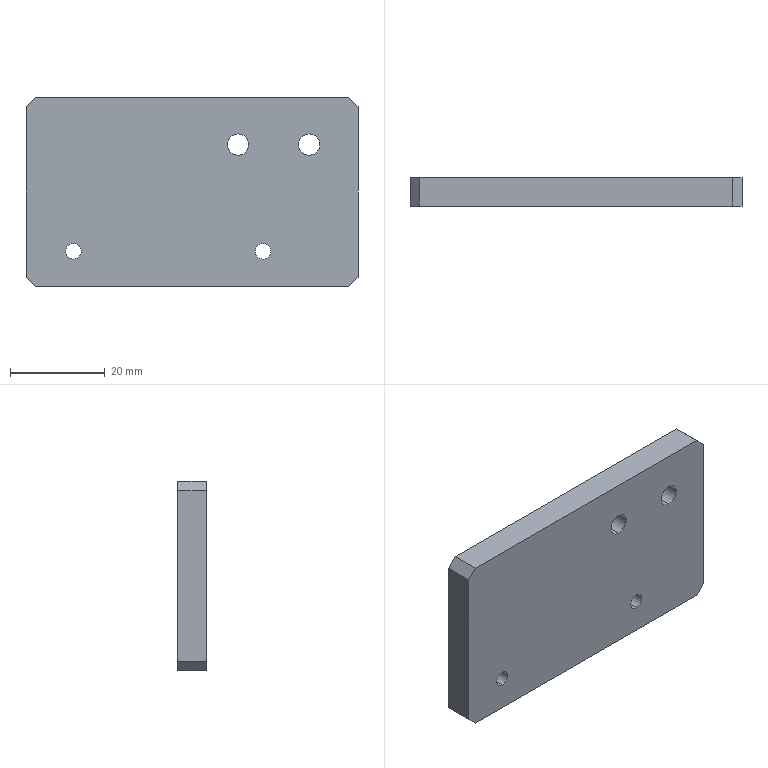Part | STEP file | PN_0023 | 1 solid | 18 faces | box 70 x 6 x 40 mm | volume 16459 mm3 | plane 10 | cylinder 8 | commonest cylinder face diameters 3.3 x4 4.5 x4
STEP:
#1=CARTESIAN_POINT('',(0.,0.,0.));
#2=DIRECTION('',(0.,0.,1.));
#3=DIRECTION('',(1.,0.,0.));
#4=AXIS2_PLACEMENT_3D('',#1,#2,#3);
#5=CARTESIAN_POINT('',(-25.,0.,-10.85));
#6=VERTEX_POINT('',#5);
#7=CARTESIAN_POINT('',(-25.,6.,-10.85));
#8=VERTEX_POINT('',#7);
#9=CARTESIAN_POINT('',(-25.,6.,-10.85));
#10=DIRECTION('',(0.,1.,0.));
#11=VECTOR('',#10,1.);
#12=LINE('',#9,#11);
#13=CARTESIAN_POINT('',(-25.,6.,-12.5));
#14=DIRECTION('',(0.,1.,0.));
#15=DIRECTION('',(0.,0.,1.));
#16=AXIS2_PLACEMENT_3D('',#13,#14,#15);
#17=CYLINDRICAL_SURFACE('',#16,1.65);
#18=CARTESIAN_POINT('',(6.283,0.));
#19=DIRECTION('',(0.,1.));
#20=VECTOR('',#19,1.);
#21=LINE('',#18,#20);
#22=(GEOMETRIC_REPRESENTATION_CONTEXT(2)PARAMETRIC_REPRESENTATION_CONTEXT()REPRESENTATION_CONTEXT('',''));
#23=DEFINITIONAL_REPRESENTATION('',(#21),#22);
#24=PCURVE('',#17,#23);
#25=CARTESIAN_POINT('',(-25.,6.,-12.5));
#26=DIRECTION('',(0.,1.,0.));
#27=DIRECTION('',(0.,0.,1.));
#28=AXIS2_PLACEMENT_3D('',#25,#26,#27);
#29=CYLINDRICAL_SURFACE('',#28,1.65);
#30=CARTESIAN_POINT('',(0.,0.));
#31=DIRECTION('',(0.,1.));
#32=VECTOR('',#31,1.);
#33=LINE('',#30,#32);
#34=(GEOMETRIC_REPRESENTATION_CONTEXT(2)PARAMETRIC_REPRESENTATION_CONTEXT()REPRESENTATION_CONTEXT('',''));
#35=DEFINITIONAL_REPRESENTATION('',(#33),#34);
#36=PCURVE('',#29,#35);
#37=SURFACE_CURVE('',#12,(#24,#36),.PCURVE_S1.);
#38=EDGE_CURVE('',#6,#8,#37,.T.);
#39=ORIENTED_EDGE('',*,*,#38,.T.);
#40=CARTESIAN_POINT('',(-25.,6.,-14.15));
#41=VERTEX_POINT('',#40);
#42=CARTESIAN_POINT('',(-25.,6.,-12.5));
#43=DIRECTION('',(0.,1.,0.));
#44=DIRECTION('',(0.,0.,1.));
#45=AXIS2_PLACEMENT_3D('',#42,#43,#44);
#46=CIRCLE('',#45,1.65);
#47=CARTESIAN_POINT('',(0.,0.));
#48=DIRECTION('',(1.,0.));
#49=VECTOR('',#48,1.);
#50=LINE('',#47,#49);
#51=(GEOMETRIC_REPRESENTATION_CONTEXT(2)PARAMETRIC_REPRESENTATION_CONTEXT()REPRESENTATION_CONTEXT('',''));
#52=DEFINITIONAL_REPRESENTATION('',(#50),#51);
#53=PCURVE('',#17,#52);
#54=CARTESIAN_POINT('',(0.,6.,0.));
#55=DIRECTION('',(0.,1.,0.));
#56=DIRECTION('',(0.,0.,1.));
#57=AXIS2_PLACEMENT_3D('',#54,#55,#56);
#58=PLANE('',#57);
#59=CARTESIAN_POINT('',(-12.5,-25.));
#60=DIRECTION('',(1.,0.));
#61=AXIS2_PLACEMENT_2D('',#59,#60);
#62=CIRCLE('',#61,1.65);
#63=(GEOMETRIC_REPRESENTATION_CONTEXT(2)PARAMETRIC_REPRESENTATION_CONTEXT()REPRESENTATION_CONTEXT('',''));
#64=DEFINITIONAL_REPRESENTATION('',(#62),#63);
#65=PCURVE('',#58,#64);
#66=SURFACE_CURVE('',#46,(#53,#65),.PCURVE_S1.);
#67=EDGE_CURVE('',#41,#8,#66,.T.);
#68=ORIENTED_EDGE('',*,*,#67,.F.);
#69=CARTESIAN_POINT('',(-25.,0.,-14.15));
#70=VERTEX_POINT('',#69);
#71=CARTESIAN_POINT('',(-25.,6.,-14.15));
#72=DIRECTION('',(0.,1.,0.));
#73=VECTOR('',#72,1.);
#74=LINE('',#71,#73);
#75=CARTESIAN_POINT('',(3.142,0.));
#76=DIRECTION('',(0.,1.));
#77=VECTOR('',#76,1.);
#78=LINE('',#75,#77);
#79=(GEOMETRIC_REPRESENTATION_CONTEXT(2)PARAMETRIC_REPRESENTATION_CONTEXT()REPRESENTATION_CONTEXT('',''));
#80=DEFINITIONAL_REPRESENTATION('',(#78),#79);
#81=PCURVE('',#17,#80);
#82=CARTESIAN_POINT('',(3.142,0.));
#83=DIRECTION('',(0.,1.));
#84=VECTOR('',#83,1.);
#85=LINE('',#82,#84);
#86=(GEOMETRIC_REPRESENTATION_CONTEXT(2)PARAMETRIC_REPRESENTATION_CONTEXT()REPRESENTATION_CONTEXT('',''));
#87=DEFINITIONAL_REPRESENTATION('',(#85),#86);
#88=PCURVE('',#29,#87);
#89=SURFACE_CURVE('',#74,(#81,#88),.PCURVE_S1.);
#90=EDGE_CURVE('',#70,#41,#89,.T.);
#91=ORIENTED_EDGE('',*,*,#90,.F.);
#92=CARTESIAN_POINT('',(-25.,0.,-12.5));
#93=DIRECTION('',(0.,1.,0.));
#94=DIRECTION('',(0.,0.,1.));
#95=AXIS2_PLACEMENT_3D('',#92,#93,#94);
#96=CIRCLE('',#95,1.65);
#97=CARTESIAN_POINT('',(0.,-6.));
#98=DIRECTION('',(1.,0.));
#99=VECTOR('',#98,1.);
#100=LINE('',#97,#99);
#101=(GEOMETRIC_REPRESENTATION_CONTEXT(2)PARAMETRIC_REPRESENTATION_CONTEXT()REPRESENTATION_CONTEXT('',''));
#102=DEFINITIONAL_REPRESENTATION('',(#100),#101);
#103=PCURVE('',#17,#102);
#104=CARTESIAN_POINT('',(0.,0.,0.));
#105=DIRECTION('',(0.,1.,0.));
#106=DIRECTION('',(0.,0.,1.));
#107=AXIS2_PLACEMENT_3D('',#104,#105,#106);
#108=PLANE('',#107);
#109=CARTESIAN_POINT('',(-12.5,-25.));
#110=DIRECTION('',(1.,0.));
#111=AXIS2_PLACEMENT_2D('',#109,#110);
#112=CIRCLE('',#111,1.65);
#113=(GEOMETRIC_REPRESENTATION_CONTEXT(2)PARAMETRIC_REPRESENTATION_CONTEXT()REPRESENTATION_CONTEXT('',''));
#114=DEFINITIONAL_REPRESENTATION('',(#112),#113);
#115=PCURVE('',#108,#114);
#116=SURFACE_CURVE('',#96,(#103,#115),.PCURVE_S1.);
#117=EDGE_CURVE('',#70,#6,#116,.T.);
#118=ORIENTED_EDGE('',*,*,#117,.T.);
#119=EDGE_LOOP('',(#39,#68,#91,#118));
#120=FACE_BOUND('',#119,.F.);
#121=ADVANCED_FACE('',(#120),#17,.F.);
#122=CARTESIAN_POINT('',(15.,0.,-10.85));
#123=VERTEX_POINT('',#122);
#124=CARTESIAN_POINT('',(15.,6.,-10.85));
#125=VERTEX_POINT('',#124);
#126=CARTESIAN_POINT('',(15.,6.,-10.85));
#127=DIRECTION('',(0.,1.,0.));
#128=VECTOR('',#127,1.);
#129=LINE('',#126,#128);
#130=CARTESIAN_POINT('',(15.,6.,-12.5));
#131=DIRECTION('',(0.,1.,0.));
#132=DIRECTION('',(0.,0.,1.));
#133=AXIS2_PLACEMENT_3D('',#130,#131,#132);
#134=CYLINDRICAL_SURFACE('',#133,1.65);
#135=CARTESIAN_POINT('',(6.283,0.));
#136=DIRECTION('',(0.,1.));
#137=VECTOR('',#136,1.);
#138=LINE('',#135,#137);
#139=(GEOMETRIC_REPRESENTATION_CONTEXT(2)PARAMETRIC_REPRESENTATION_CONTEXT()REPRESENTATION_CONTEXT('',''));
#140=DEFINITIONAL_REPRESENTATION('',(#138),#139);
#141=PCURVE('',#134,#140);
#142=CARTESIAN_POINT('',(15.,6.,-12.5));
#143=DIRECTION('',(0.,1.,0.));
#144=DIRECTION('',(0.,0.,1.));
#145=AXIS2_PLACEMENT_3D('',#142,#143,#144);
#146=CYLINDRICAL_SURFACE('',#145,1.65);
#147=CARTESIAN_POINT('',(0.,0.));
#148=DIRECTION('',(0.,1.));
#149=VECTOR('',#148,1.);
#150=LINE('',#147,#149);
#151=(GEOMETRIC_REPRESENTATION_CONTEXT(2)PARAMETRIC_REPRESENTATION_CONTEXT()REPRESENTATION_CONTEXT('',''));
#152=DEFINITIONAL_REPRESENTATION('',(#150),#151);
#153=PCURVE('',#146,#152);
#154=SURFACE_CURVE('',#129,(#141,#153),.PCURVE_S1.);
#155=EDGE_CURVE('',#123,#125,#154,.T.);
#156=ORIENTED_EDGE('',*,*,#155,.T.);
#157=CARTESIAN_POINT('',(15.,6.,-14.15));
#158=VERTEX_POINT('',#157);
#159=CARTESIAN_POINT('',(15.,6.,-12.5));
#160=DIRECTION('',(0.,1.,0.));
#161=DIRECTION('',(0.,0.,1.));
#162=AXIS2_PLACEMENT_3D('',#159,#160,#161);
#163=CIRCLE('',#162,1.65);
#164=CARTESIAN_POINT('',(0.,0.));
#165=DIRECTION('',(1.,0.));
#166=VECTOR('',#165,1.);
#167=LINE('',#164,#166);
#168=(GEOMETRIC_REPRESENTATION_CONTEXT(2)PARAMETRIC_REPRESENTATION_CONTEXT()REPRESENTATION_CONTEXT('',''));
#169=DEFINITIONAL_REPRESENTATION('',(#167),#168);
#170=PCURVE('',#134,#169);
#171=CARTESIAN_POINT('',(-12.5,15.));
#172=DIRECTION('',(1.,0.));
#173=AXIS2_PLACEMENT_2D('',#171,#172);
#174=CIRCLE('',#173,1.65);
#175=(GEOMETRIC_REPRESENTATION_CONTEXT(2)PARAMETRIC_REPRESENTATION_CONTEXT()REPRESENTATION_CONTEXT('',''));
#176=DEFINITIONAL_REPRESENTATION('',(#174),#175);
#177=PCURVE('',#58,#176);
#178=SURFACE_CURVE('',#163,(#170,#177),.PCURVE_S1.);
#179=EDGE_CURVE('',#158,#125,#178,.T.);
#180=ORIENTED_EDGE('',*,*,#179,.F.);
#181=CARTESIAN_POINT('',(15.,0.,-14.15));
#182=VERTEX_POINT('',#181);
#183=CARTESIAN_POINT('',(15.,6.,-14.15));
#184=DIRECTION('',(0.,1.,0.));
#185=VECTOR('',#184,1.);
#186=LINE('',#183,#185);
#187=CARTESIAN_POINT('',(3.142,0.));
#188=DIRECTION('',(0.,1.));
#189=VECTOR('',#188,1.);
#190=LINE('',#187,#189);
#191=(GEOMETRIC_REPRESENTATION_CONTEXT(2)PARAMETRIC_REPRESENTATION_CONTEXT()REPRESENTATION_CONTEXT('',''));
#192=DEFINITIONAL_REPRESENTATION('',(#190),#191);
#193=PCURVE('',#134,#192);
#194=CARTESIAN_POINT('',(3.142,0.));
#195=DIRECTION('',(0.,1.));
#196=VECTOR('',#195,1.);
#197=LINE('',#194,#196);
#198=(GEOMETRIC_REPRESENTATION_CONTEXT(2)PARAMETRIC_REPRESENTATION_CONTEXT()REPRESENTATION_CONTEXT('',''));
#199=DEFINITIONAL_REPRESENTATION('',(#197),#198);
#200=PCURVE('',#146,#199);
#201=SURFACE_CURVE('',#186,(#193,#200),.PCURVE_S1.);
#202=EDGE_CURVE('',#182,#158,#201,.T.);
#203=ORIENTED_EDGE('',*,*,#202,.F.);
#204=CARTESIAN_POINT('',(15.,0.,-12.5));
#205=DIRECTION('',(0.,1.,0.));
#206=DIRECTION('',(0.,0.,1.));
#207=AXIS2_PLACEMENT_3D('',#204,#205,#206);
#208=CIRCLE('',#207,1.65);
#209=CARTESIAN_POINT('',(0.,-6.));
#210=DIRECTION('',(1.,0.));
#211=VECTOR('',#210,1.);
#212=LINE('',#209,#211);
#213=(GEOMETRIC_REPRESENTATION_CONTEXT(2)PARAMETRIC_REPRESENTATION_CONTEXT()REPRESENTATION_CONTEXT('',''));
#214=DEFINITIONAL_REPRESENTATION('',(#212),#213);
#215=PCURVE('',#134,#214);
#216=CARTESIAN_POINT('',(-12.5,15.));
#217=DIRECTION('',(1.,0.));
#218=AXIS2_PLACEMENT_2D('',#216,#217);
#219=CIRCLE('',#218,1.65);
#220=(GEOMETRIC_REPRESENTATION_CONTEXT(2)PARAMETRIC_REPRESENTATION_CONTEXT()REPRESENTATION_CONTEXT('',''));
#221=DEFINITIONAL_REPRESENTATION('',(#219),#220);
#222=PCURVE('',#108,#221);
#223=SURFACE_CURVE('',#208,(#215,#222),.PCURVE_S1.);
#224=EDGE_CURVE('',#182,#123,#223,.T.);
#225=ORIENTED_EDGE('',*,*,#224,.T.);
#226=EDGE_LOOP('',(#156,#180,#203,#225));
#227=FACE_BOUND('',#226,.F.);
#228=ADVANCED_FACE('',(#227),#134,.F.);
#229=CARTESIAN_POINT('',(24.703,0.,12.25));
#230=VERTEX_POINT('',#229);
#231=CARTESIAN_POINT('',(24.703,6.,12.25));
#232=VERTEX_POINT('',#231);
#233=CARTESIAN_POINT('',(24.703,6.,12.25));
#234=DIRECTION('',(0.,1.,0.));
#235=VECTOR('',#234,1.);
#236=LINE('',#233,#235);
#237=CARTESIAN_POINT('',(24.703,6.,10.));
#238=DIRECTION('',(0.,1.,0.));
#239=DIRECTION('',(0.,0.,1.));
#240=AXIS2_PLACEMENT_3D('',#237,#238,#239);
#241=CYLINDRICAL_SURFACE('',#240,2.25);
#242=CARTESIAN_POINT('',(6.283,0.));
#243=DIRECTION('',(0.,1.));
#244=VECTOR('',#243,1.);
#245=LINE('',#242,#244);
#246=(GEOMETRIC_REPRESENTATION_CONTEXT(2)PARAMETRIC_REPRESENTATION_CONTEXT()REPRESENTATION_CONTEXT('',''));
#247=DEFINITIONAL_REPRESENTATION('',(#245),#246);
#248=PCURVE('',#241,#247);
#249=CARTESIAN_POINT('',(24.703,6.,10.));
#250=DIRECTION('',(0.,1.,0.));
#251=DIRECTION('',(0.,0.,1.));
#252=AXIS2_PLACEMENT_3D('',#249,#250,#251);
#253=CYLINDRICAL_SURFACE('',#252,2.25);
#254=CARTESIAN_POINT('',(0.,0.));
#255=DIRECTION('',(0.,1.));
#256=VECTOR('',#255,1.);
#257=LINE('',#254,#256);
#258=(GEOMETRIC_REPRESENTATION_CONTEXT(2)PARAMETRIC_REPRESENTATION_CONTEXT()REPRESENTATION_CONTEXT('',''));
#259=DEFINITIONAL_REPRESENTATION('',(#257),#258);
#260=PCURVE('',#253,#259);
#261=SURFACE_CURVE('',#236,(#248,#260),.PCURVE_S1.);
#262=EDGE_CURVE('',#230,#232,#261,.T.);
#263=ORIENTED_EDGE('',*,*,#262,.T.);
#264=CARTESIAN_POINT('',(24.703,6.,7.75));
#265=VERTEX_POINT('',#264);
#266=CARTESIAN_POINT('',(24.703,6.,10.));
#267=DIRECTION('',(0.,1.,0.));
#268=DIRECTION('',(0.,0.,1.));
#269=AXIS2_PLACEMENT_3D('',#266,#267,#268);
#270=CIRCLE('',#269,2.25);
#271=CARTESIAN_POINT('',(0.,0.));
#272=DIRECTION('',(1.,0.));
#273=VECTOR('',#272,1.);
#274=LINE('',#271,#273);
#275=(GEOMETRIC_REPRESENTATION_CONTEXT(2)PARAMETRIC_REPRESENTATION_CONTEXT()REPRESENTATION_CONTEXT('',''));
#276=DEFINITIONAL_REPRESENTATION('',(#274),#275);
#277=PCURVE('',#241,#276);
#278=CARTESIAN_POINT('',(10.,24.703));
#279=DIRECTION('',(1.,0.));
#280=AXIS2_PLACEMENT_2D('',#278,#279);
#281=CIRCLE('',#280,2.25);
#282=(GEOMETRIC_REPRESENTATION_CONTEXT(2)PARAMETRIC_REPRESENTATION_CONTEXT()REPRESENTATION_CONTEXT('',''));
#283=DEFINITIONAL_REPRESENTATION('',(#281),#282);
#284=PCURVE('',#58,#283);
#285=SURFACE_CURVE('',#270,(#277,#284),.PCURVE_S1.);
#286=EDGE_CURVE('',#265,#232,#285,.T.);
#287=ORIENTED_EDGE('',*,*,#286,.F.);
#288=CARTESIAN_POINT('',(24.703,0.,7.75));
#289=VERTEX_POINT('',#288);
#290=CARTESIAN_POINT('',(24.703,6.,7.75));
#291=DIRECTION('',(0.,1.,0.));
#292=VECTOR('',#291,1.);
#293=LINE('',#290,#292);
#294=CARTESIAN_POINT('',(3.142,0.));
#295=DIRECTION('',(0.,1.));
#296=VECTOR('',#295,1.);
#297=LINE('',#294,#296);
#298=(GEOMETRIC_REPRESENTATION_CONTEXT(2)PARAMETRIC_REPRESENTATION_CONTEXT()REPRESENTATION_CONTEXT('',''));
#299=DEFINITIONAL_REPRESENTATION('',(#297),#298);
#300=PCURVE('',#241,#299);
#301=CARTESIAN_POINT('',(3.142,0.));
#302=DIRECTION('',(0.,1.));
#303=VECTOR('',#302,1.);
#304=LINE('',#301,#303);
#305=(GEOMETRIC_REPRESENTATION_CONTEXT(2)PARAMETRIC_REPRESENTATION_CONTEXT()REPRESENTATION_CONTEXT('',''));
#306=DEFINITIONAL_REPRESENTATION('',(#304),#305);
#307=PCURVE('',#253,#306);
#308=SURFACE_CURVE('',#293,(#300,#307),.PCURVE_S1.);
#309=EDGE_CURVE('',#289,#265,#308,.T.);
#310=ORIENTED_EDGE('',*,*,#309,.F.);
#311=CARTESIAN_POINT('',(24.703,0.,10.));
#312=DIRECTION('',(0.,1.,0.));
#313=DIRECTION('',(0.,0.,1.));
#314=AXIS2_PLACEMENT_3D('',#311,#312,#313);
#315=CIRCLE('',#314,2.25);
#316=CARTESIAN_POINT('',(0.,-6.));
#317=DIRECTION('',(1.,0.));
#318=VECTOR('',#317,1.);
#319=LINE('',#316,#318);
#320=(GEOMETRIC_REPRESENTATION_CONTEXT(2)PARAMETRIC_REPRESENTATION_CONTEXT()REPRESENTATION_CONTEXT('',''));
#321=DEFINITIONAL_REPRESENTATION('',(#319),#320);
#322=PCURVE('',#241,#321);
#323=CARTESIAN_POINT('',(10.,24.703));
#324=DIRECTION('',(1.,0.));
#325=AXIS2_PLACEMENT_2D('',#323,#324);
#326=CIRCLE('',#325,2.25);
#327=(GEOMETRIC_REPRESENTATION_CONTEXT(2)PARAMETRIC_REPRESENTATION_CONTEXT()REPRESENTATION_CONTEXT('',''));
#328=DEFINITIONAL_REPRESENTATION('',(#326),#327);
#329=PCURVE('',#108,#328);
#330=SURFACE_CURVE('',#315,(#322,#329),.PCURVE_S1.);
#331=EDGE_CURVE('',#289,#230,#330,.T.);
#332=ORIENTED_EDGE('',*,*,#331,.T.);
#333=EDGE_LOOP('',(#263,#287,#310,#332));
#334=FACE_BOUND('',#333,.F.);
#335=ADVANCED_FACE('',(#334),#241,.F.);
#336=CARTESIAN_POINT('',(9.703,0.,12.25));
#337=VERTEX_POINT('',#336);
#338=CARTESIAN_POINT('',(9.703,6.,12.25));
#339=VERTEX_POINT('',#338);
#340=CARTESIAN_POINT('',(9.703,6.,12.25));
#341=DIRECTION('',(0.,1.,0.));
#342=VECTOR('',#341,1.);
#343=LINE('',#340,#342);
#344=CARTESIAN_POINT('',(9.703,6.,10.));
#345=DIRECTION('',(0.,1.,0.));
#346=DIRECTION('',(0.,0.,1.));
#347=AXIS2_PLACEMENT_3D('',#344,#345,#346);
#348=CYLINDRICAL_SURFACE('',#347,2.25);
#349=CARTESIAN_POINT('',(6.283,0.));
#350=DIRECTION('',(0.,1.));
#351=VECTOR('',#350,1.);
#352=LINE('',#349,#351);
#353=(GEOMETRIC_REPRESENTATION_CONTEXT(2)PARAMETRIC_REPRESENTATION_CONTEXT()REPRESENTATION_CONTEXT('',''));
#354=DEFINITIONAL_REPRESENTATION('',(#352),#353);
#355=PCURVE('',#348,#354);
#356=CARTESIAN_POINT('',(9.703,6.,10.));
#357=DIRECTION('',(0.,1.,0.));
#358=DIRECTION('',(0.,0.,1.));
#359=AXIS2_PLACEMENT_3D('',#356,#357,#358);
#360=CYLINDRICAL_SURFACE('',#359,2.25);
#361=CARTESIAN_POINT('',(0.,0.));
#362=DIRECTION('',(0.,1.));
#363=VECTOR('',#362,1.);
#364=LINE('',#361,#363);
#365=(GEOMETRIC_REPRESENTATION_CONTEXT(2)PARAMETRIC_REPRESENTATION_CONTEXT()REPRESENTATION_CONTEXT('',''));
#366=DEFINITIONAL_REPRESENTATION('',(#364),#365);
#367=PCURVE('',#360,#366);
#368=SURFACE_CURVE('',#343,(#355,#367),.PCURVE_S1.);
#369=EDGE_CURVE('',#337,#339,#368,.T.);
#370=ORIENTED_EDGE('',*,*,#369,.T.);
#371=CARTESIAN_POINT('',(9.703,6.,7.75));
#372=VERTEX_POINT('',#371);
#373=CARTESIAN_POINT('',(9.703,6.,10.));
#374=DIRECTION('',(0.,1.,0.));
#375=DIRECTION('',(0.,0.,1.));
#376=AXIS2_PLACEMENT_3D('',#373,#374,#375);
#377=CIRCLE('',#376,2.25);
#378=CARTESIAN_POINT('',(0.,0.));
#379=DIRECTION('',(1.,0.));
#380=VECTOR('',#379,1.);
#381=LINE('',#378,#380);
#382=(GEOMETRIC_REPRESENTATION_CONTEXT(2)PARAMETRIC_REPRESENTATION_CONTEXT()REPRESENTATION_CONTEXT('',''));
#383=DEFINITIONAL_REPRESENTATION('',(#381),#382);
#384=PCURVE('',#348,#383);
#385=CARTESIAN_POINT('',(10.,9.703));
#386=DIRECTION('',(1.,0.));
#387=AXIS2_PLACEMENT_2D('',#385,#386);
#388=CIRCLE('',#387,2.25);
#389=(GEOMETRIC_REPRESENTATION_CONTEXT(2)PARAMETRIC_REPRESENTATION_CONTEXT()REPRESENTATION_CONTEXT('',''));
#390=DEFINITIONAL_REPRESENTATION('',(#388),#389);
#391=PCURVE('',#58,#390);
#392=SURFACE_CURVE('',#377,(#384,#391),.PCURVE_S1.);
#393=EDGE_CURVE('',#372,#339,#392,.T.);
#394=ORIENTED_EDGE('',*,*,#393,.F.);
#395=CARTESIAN_POINT('',(9.703,0.,7.75));
#396=VERTEX_POINT('',#395);
#397=CARTESIAN_POINT('',(9.703,6.,7.75));
#398=DIRECTION('',(0.,1.,0.));
#399=VECTOR('',#398,1.);
#400=LINE('',#397,#399);
#401=CARTESIAN_POINT('',(3.142,0.));
#402=DIRECTION('',(0.,1.));
#403=VECTOR('',#402,1.);
#404=LINE('',#401,#403);
#405=(GEOMETRIC_REPRESENTATION_CONTEXT(2)PARAMETRIC_REPRESENTATION_CONTEXT()REPRESENTATION_CONTEXT('',''));
#406=DEFINITIONAL_REPRESENTATION('',(#404),#405);
#407=PCURVE('',#348,#406);
#408=CARTESIAN_POINT('',(3.142,0.));
#409=DIRECTION('',(0.,1.));
#410=VECTOR('',#409,1.);
#411=LINE('',#408,#410);
#412=(GEOMETRIC_REPRESENTATION_CONTEXT(2)PARAMETRIC_REPRESENTATION_CONTEXT()REPRESENTATION_CONTEXT('',''));
#413=DEFINITIONAL_REPRESENTATION('',(#411),#412);
#414=PCURVE('',#360,#413);
#415=SURFACE_CURVE('',#400,(#407,#414),.PCURVE_S1.);
#416=EDGE_CURVE('',#396,#372,#415,.T.);
#417=ORIENTED_EDGE('',*,*,#416,.F.);
#418=CARTESIAN_POINT('',(9.703,0.,10.));
#419=DIRECTION('',(0.,1.,0.));
#420=DIRECTION('',(0.,0.,1.));
#421=AXIS2_PLACEMENT_3D('',#418,#419,#420);
#422=CIRCLE('',#421,2.25);
#423=CARTESIAN_POINT('',(0.,-6.));
#424=DIRECTION('',(1.,0.));
#425=VECTOR('',#424,1.);
#426=LINE('',#423,#425);
#427=(GEOMETRIC_REPRESENTATION_CONTEXT(2)PARAMETRIC_REPRESENTATION_CONTEXT()REPRESENTATION_CONTEXT('',''));
#428=DEFINITIONAL_REPRESENTATION('',(#426),#427);
#429=PCURVE('',#348,#428);
#430=CARTESIAN_POINT('',(10.,9.703));
#431=DIRECTION('',(1.,0.));
#432=AXIS2_PLACEMENT_2D('',#430,#431);
#433=CIRCLE('',#432,2.25);
#434=(GEOMETRIC_REPRESENTATION_CONTEXT(2)PARAMETRIC_REPRESENTATION_CONTEXT()REPRESENTATION_CONTEXT('',''));
#435=DEFINITIONAL_REPRESENTATION('',(#433),#434);
#436=PCURVE('',#108,#435);
#437=SURFACE_CURVE('',#422,(#429,#436),.PCURVE_S1.);
#438=EDGE_CURVE('',#396,#337,#437,.T.);
#439=ORIENTED_EDGE('',*,*,#438,.T.);
#440=EDGE_LOOP('',(#370,#394,#417,#439));
#441=FACE_BOUND('',#440,.F.);
#442=ADVANCED_FACE('',(#441),#348,.F.);
#443=CARTESIAN_POINT('',(35.,6.,18.));
#444=VERTEX_POINT('',#443);
#445=CARTESIAN_POINT('',(35.,6.,-18.));
#446=VERTEX_POINT('',#445);
#447=CARTESIAN_POINT('',(35.,6.,-20.));
#448=DIRECTION('',(0.,0.,-1.));
#449=VECTOR('',#448,1.);
#450=LINE('',#447,#449);
#451=CARTESIAN_POINT('',(35.,6.,-20.));
#452=DIRECTION('',(-1.,0.,0.));
#453=DIRECTION('',(0.,0.,1.));
#454=AXIS2_PLACEMENT_3D('',#451,#452,#453);
#455=PLANE('',#454);
#456=CARTESIAN_POINT('',(0.,0.));
#457=DIRECTION('',(-1.,0.));
#458=VECTOR('',#457,1.);
#459=LINE('',#456,#458);
#460=(GEOMETRIC_REPRESENTATION_CONTEXT(2)PARAMETRIC_REPRESENTATION_CONTEXT()REPRESENTATION_CONTEXT('',''));
#461=DEFINITIONAL_REPRESENTATION('',(#459),#460);
#462=PCURVE('',#455,#461);
#463=CARTESIAN_POINT('',(-20.,35.));
#464=DIRECTION('',(-1.,0.));
#465=VECTOR('',#464,1.);
#466=LINE('',#463,#465);
#467=(GEOMETRIC_REPRESENTATION_CONTEXT(2)PARAMETRIC_REPRESENTATION_CONTEXT()REPRESENTATION_CONTEXT('',''));
#468=DEFINITIONAL_REPRESENTATION('',(#466),#467);
#469=PCURVE('',#58,#468);
#470=SURFACE_CURVE('',#450,(#462,#469),.PCURVE_S1.);
#471=EDGE_CURVE('',#444,#446,#470,.T.);
#472=ORIENTED_EDGE('',*,*,#471,.F.);
#473=CARTESIAN_POINT('',(35.,0.,18.));
#474=VERTEX_POINT('',#473);
#475=CARTESIAN_POINT('',(35.,6.,18.));
#476=DIRECTION('',(0.,-1.,0.));
#477=VECTOR('',#476,1.);
#478=LINE('',#475,#477);
#479=CARTESIAN_POINT('',(38.,0.));
#480=DIRECTION('',(0.,-1.));
#481=VECTOR('',#480,1.);
#482=LINE('',#479,#481);
#483=(GEOMETRIC_REPRESENTATION_CONTEXT(2)PARAMETRIC_REPRESENTATION_CONTEXT()REPRESENTATION_CONTEXT('',''));
#484=DEFINITIONAL_REPRESENTATION('',(#482),#483);
#485=PCURVE('',#455,#484);
#486=CARTESIAN_POINT('',(35.,6.,18.));
#487=DIRECTION('',(-0.7071,0.,-0.7071));
#488=DIRECTION('',(0.,-1.,0.));
#489=AXIS2_PLACEMENT_3D('',#486,#487,#488);
#490=PLANE('',#489);
#491=CARTESIAN_POINT('',(0.,0.));
#492=DIRECTION('',(1.,0.));
#493=VECTOR('',#492,1.);
#494=LINE('',#491,#493);
#495=(GEOMETRIC_REPRESENTATION_CONTEXT(2)PARAMETRIC_REPRESENTATION_CONTEXT()REPRESENTATION_CONTEXT('',''));
#496=DEFINITIONAL_REPRESENTATION('',(#494),#495);
#497=PCURVE('',#490,#496);
#498=SURFACE_CURVE('',#478,(#485,#497),.PCURVE_S1.);
#499=EDGE_CURVE('',#444,#474,#498,.T.);
#500=ORIENTED_EDGE('',*,*,#499,.T.);
#501=CARTESIAN_POINT('',(35.,0.,-18.));
#502=VERTEX_POINT('',#501);
#503=CARTESIAN_POINT('',(35.,0.,-20.));
#504=DIRECTION('',(0.,0.,-1.));
#505=VECTOR('',#504,1.);
#506=LINE('',#503,#505);
#507=CARTESIAN_POINT('',(0.,-6.));
#508=DIRECTION('',(-1.,0.));
#509=VECTOR('',#508,1.);
#510=LINE('',#507,#509);
#511=(GEOMETRIC_REPRESENTATION_CONTEXT(2)PARAMETRIC_REPRESENTATION_CONTEXT()REPRESENTATION_CONTEXT('',''));
#512=DEFINITIONAL_REPRESENTATION('',(#510),#511);
#513=PCURVE('',#455,#512);
#514=CARTESIAN_POINT('',(-20.,35.));
#515=DIRECTION('',(-1.,0.));
#516=VECTOR('',#515,1.);
#517=LINE('',#514,#516);
#518=(GEOMETRIC_REPRESENTATION_CONTEXT(2)PARAMETRIC_REPRESENTATION_CONTEXT()REPRESENTATION_CONTEXT('',''));
#519=DEFINITIONAL_REPRESENTATION('',(#517),#518);
#520=PCURVE('',#108,#519);
#521=SURFACE_CURVE('',#506,(#513,#520),.PCURVE_S1.);
#522=EDGE_CURVE('',#474,#502,#521,.T.);
#523=ORIENTED_EDGE('',*,*,#522,.T.);
#524=CARTESIAN_POINT('',(35.,6.,-18.));
#525=DIRECTION('',(0.,1.,0.));
#526=VECTOR('',#525,1.);
#527=LINE('',#524,#526);
#528=CARTESIAN_POINT('',(2.,0.));
#529=DIRECTION('',(0.,1.));
#530=VECTOR('',#529,1.);
#531=LINE('',#528,#530);
#532=(GEOMETRIC_REPRESENTATION_CONTEXT(2)PARAMETRIC_REPRESENTATION_CONTEXT()REPRESENTATION_CONTEXT('',''));
#533=DEFINITIONAL_REPRESENTATION('',(#531),#532);
#534=PCURVE('',#455,#533);
#535=CARTESIAN_POINT('',(33.,6.,-20.));
#536=DIRECTION('',(-0.7071,0.,0.7071));
#537=DIRECTION('',(0.,-1.,0.));
#538=AXIS2_PLACEMENT_3D('',#535,#536,#537);
#539=PLANE('',#538);
#540=CARTESIAN_POINT('',(0.,2.828));
#541=DIRECTION('',(-1.,0.));
#542=VECTOR('',#541,1.);
#543=LINE('',#540,#542);
#544=(GEOMETRIC_REPRESENTATION_CONTEXT(2)PARAMETRIC_REPRESENTATION_CONTEXT()REPRESENTATION_CONTEXT('',''));
#545=DEFINITIONAL_REPRESENTATION('',(#543),#544);
#546=PCURVE('',#539,#545);
#547=SURFACE_CURVE('',#527,(#534,#546),.PCURVE_S1.);
#548=EDGE_CURVE('',#502,#446,#547,.T.);
#549=ORIENTED_EDGE('',*,*,#548,.T.);
#550=EDGE_LOOP('',(#472,#500,#523,#549));
#551=FACE_BOUND('',#550,.T.);
#552=ADVANCED_FACE('',(#551),#455,.F.);
#553=CARTESIAN_POINT('',(33.,0.,-20.));
#554=VERTEX_POINT('',#553);
#555=CARTESIAN_POINT('',(-33.,0.,-20.));
#556=VERTEX_POINT('',#555);
#557=CARTESIAN_POINT('',(-35.,0.,-20.));
#558=DIRECTION('',(-1.,0.,0.));
#559=VECTOR('',#558,1.);
#560=LINE('',#557,#559);
#561=CARTESIAN_POINT('',(-35.,6.,-20.));
#562=DIRECTION('',(0.,0.,1.));
#563=DIRECTION('',(1.,0.,0.));
#564=AXIS2_PLACEMENT_3D('',#561,#562,#563);
#565=PLANE('',#564);
#566=CARTESIAN_POINT('',(0.,-6.));
#567=DIRECTION('',(-1.,0.));
#568=VECTOR('',#567,1.);
#569=LINE('',#566,#568);
#570=(GEOMETRIC_REPRESENTATION_CONTEXT(2)PARAMETRIC_REPRESENTATION_CONTEXT()REPRESENTATION_CONTEXT('',''));
#571=DEFINITIONAL_REPRESENTATION('',(#569),#570);
#572=PCURVE('',#565,#571);
#573=CARTESIAN_POINT('',(-20.,-35.));
#574=DIRECTION('',(0.,-1.));
#575=VECTOR('',#574,1.);
#576=LINE('',#573,#575);
#577=(GEOMETRIC_REPRESENTATION_CONTEXT(2)PARAMETRIC_REPRESENTATION_CONTEXT()REPRESENTATION_CONTEXT('',''));
#578=DEFINITIONAL_REPRESENTATION('',(#576),#577);
#579=PCURVE('',#108,#578);
#580=SURFACE_CURVE('',#560,(#572,#579),.PCURVE_S1.);
#581=EDGE_CURVE('',#554,#556,#580,.T.);
#582=ORIENTED_EDGE('',*,*,#581,.T.);
#583=CARTESIAN_POINT('',(-33.,6.,-20.));
#584=VERTEX_POINT('',#583);
#585=CARTESIAN_POINT('',(-33.,6.,-20.));
#586=DIRECTION('',(0.,1.,0.));
#587=VECTOR('',#586,1.);
#588=LINE('',#585,#587);
#589=CARTESIAN_POINT('',(2.,0.));
#590=DIRECTION('',(0.,1.));
#591=VECTOR('',#590,1.);
#592=LINE('',#589,#591);
#593=(GEOMETRIC_REPRESENTATION_CONTEXT(2)PARAMETRIC_REPRESENTATION_CONTEXT()REPRESENTATION_CONTEXT('',''));
#594=DEFINITIONAL_REPRESENTATION('',(#592),#593);
#595=PCURVE('',#565,#594);
#596=CARTESIAN_POINT('',(-35.,6.,-18.));
#597=DIRECTION('',(0.7071,0.,0.7071));
#598=DIRECTION('',(0.,-1.,0.));
#599=AXIS2_PLACEMENT_3D('',#596,#597,#598);
#600=PLANE('',#599);
#601=CARTESIAN_POINT('',(0.,2.828));
#602=DIRECTION('',(-1.,0.));
#603=VECTOR('',#602,1.);
#604=LINE('',#601,#603);
#605=(GEOMETRIC_REPRESENTATION_CONTEXT(2)PARAMETRIC_REPRESENTATION_CONTEXT()REPRESENTATION_CONTEXT('',''));
#606=DEFINITIONAL_REPRESENTATION('',(#604),#605);
#607=PCURVE('',#600,#606);
#608=SURFACE_CURVE('',#588,(#595,#607),.PCURVE_S1.);
#609=EDGE_CURVE('',#556,#584,#608,.T.);
#610=ORIENTED_EDGE('',*,*,#609,.T.);
#611=CARTESIAN_POINT('',(33.,6.,-20.));
#612=VERTEX_POINT('',#611);
#613=CARTESIAN_POINT('',(-35.,6.,-20.));
#614=DIRECTION('',(-1.,0.,0.));
#615=VECTOR('',#614,1.);
#616=LINE('',#613,#615);
#617=CARTESIAN_POINT('',(0.,0.));
#618=DIRECTION('',(-1.,0.));
#619=VECTOR('',#618,1.);
#620=LINE('',#617,#619);
#621=(GEOMETRIC_REPRESENTATION_CONTEXT(2)PARAMETRIC_REPRESENTATION_CONTEXT()REPRESENTATION_CONTEXT('',''));
#622=DEFINITIONAL_REPRESENTATION('',(#620),#621);
#623=PCURVE('',#565,#622);
#624=CARTESIAN_POINT('',(-20.,-35.));
#625=DIRECTION('',(0.,-1.));
#626=VECTOR('',#625,1.);
#627=LINE('',#624,#626);
#628=(GEOMETRIC_REPRESENTATION_CONTEXT(2)PARAMETRIC_REPRESENTATION_CONTEXT()REPRESENTATION_CONTEXT('',''));
#629=DEFINITIONAL_REPRESENTATION('',(#627),#628);
#630=PCURVE('',#58,#629);
#631=SURFACE_CURVE('',#616,(#623,#630),.PCURVE_S1.);
#632=EDGE_CURVE('',#612,#584,#631,.T.);
#633=ORIENTED_EDGE('',*,*,#632,.F.);
#634=CARTESIAN_POINT('',(33.,6.,-20.));
#635=DIRECTION('',(0.,-1.,0.));
#636=VECTOR('',#635,1.);
#637=LINE('',#634,#636);
#638=CARTESIAN_POINT('',(68.,0.));
#639=DIRECTION('',(0.,-1.));
#640=VECTOR('',#639,1.);
#641=LINE('',#638,#640);
#642=(GEOMETRIC_REPRESENTATION_CONTEXT(2)PARAMETRIC_REPRESENTATION_CONTEXT()REPRESENTATION_CONTEXT('',''));
#643=DEFINITIONAL_REPRESENTATION('',(#641),#642);
#644=PCURVE('',#565,#643);
#645=CARTESIAN_POINT('',(0.,0.));
#646=DIRECTION('',(1.,0.));
#647=VECTOR('',#646,1.);
#648=LINE('',#645,#647);
#649=(GEOMETRIC_REPRESENTATION_CONTEXT(2)PARAMETRIC_REPRESENTATION_CONTEXT()REPRESENTATION_CONTEXT('',''));
#650=DEFINITIONAL_REPRESENTATION('',(#648),#649);
#651=PCURVE('',#539,#650);
#652=SURFACE_CURVE('',#637,(#644,#651),.PCURVE_S1.);
#653=EDGE_CURVE('',#612,#554,#652,.T.);
#654=ORIENTED_EDGE('',*,*,#653,.T.);
#655=EDGE_LOOP('',(#582,#610,#633,#654));
#656=FACE_BOUND('',#655,.T.);
#657=ADVANCED_FACE('',(#656),#565,.F.);
#658=CARTESIAN_POINT('',(-35.,6.,-18.));
#659=VERTEX_POINT('',#658);
#660=CARTESIAN_POINT('',(-35.,6.,18.));
#661=VERTEX_POINT('',#660);
#662=CARTESIAN_POINT('',(-35.,6.,-20.));
#663=DIRECTION('',(0.,0.,1.));
#664=VECTOR('',#663,1.);
#665=LINE('',#662,#664);
#666=CARTESIAN_POINT('',(-35.,6.,-20.));
#667=DIRECTION('',(1.,0.,0.));
#668=DIRECTION('',(0.,0.,-1.));
#669=AXIS2_PLACEMENT_3D('',#666,#667,#668);
#670=PLANE('',#669);
#671=CARTESIAN_POINT('',(0.,0.));
#672=DIRECTION('',(-1.,0.));
#673=VECTOR('',#672,1.);
#674=LINE('',#671,#673);
#675=(GEOMETRIC_REPRESENTATION_CONTEXT(2)PARAMETRIC_REPRESENTATION_CONTEXT()REPRESENTATION_CONTEXT('',''));
#676=DEFINITIONAL_REPRESENTATION('',(#674),#675);
#677=PCURVE('',#670,#676);
#678=CARTESIAN_POINT('',(-20.,-35.));
#679=DIRECTION('',(1.,0.));
#680=VECTOR('',#679,1.);
#681=LINE('',#678,#680);
#682=(GEOMETRIC_REPRESENTATION_CONTEXT(2)PARAMETRIC_REPRESENTATION_CONTEXT()REPRESENTATION_CONTEXT('',''));
#683=DEFINITIONAL_REPRESENTATION('',(#681),#682);
#684=PCURVE('',#58,#683);
#685=SURFACE_CURVE('',#665,(#677,#684),.PCURVE_S1.);
#686=EDGE_CURVE('',#659,#661,#685,.T.);
#687=ORIENTED_EDGE('',*,*,#686,.F.);
#688=CARTESIAN_POINT('',(-35.,0.,-18.));
#689=VERTEX_POINT('',#688);
#690=CARTESIAN_POINT('',(-35.,6.,-18.));
#691=DIRECTION('',(0.,-1.,0.));
#692=VECTOR('',#691,1.);
#693=LINE('',#690,#692);
#694=CARTESIAN_POINT('',(-2.,0.));
#695=DIRECTION('',(0.,-1.));
#696=VECTOR('',#695,1.);
#697=LINE('',#694,#696);
#698=(GEOMETRIC_REPRESENTATION_CONTEXT(2)PARAMETRIC_REPRESENTATION_CONTEXT()REPRESENTATION_CONTEXT('',''));
#699=DEFINITIONAL_REPRESENTATION('',(#697),#698);
#700=PCURVE('',#670,#699);
#701=CARTESIAN_POINT('',(0.,0.));
#702=DIRECTION('',(1.,0.));
#703=VECTOR('',#702,1.);
#704=LINE('',#701,#703);
#705=(GEOMETRIC_REPRESENTATION_CONTEXT(2)PARAMETRIC_REPRESENTATION_CONTEXT()REPRESENTATION_CONTEXT('',''));
#706=DEFINITIONAL_REPRESENTATION('',(#704),#705);
#707=PCURVE('',#600,#706);
#708=SURFACE_CURVE('',#693,(#700,#707),.PCURVE_S1.);
#709=EDGE_CURVE('',#659,#689,#708,.T.);
#710=ORIENTED_EDGE('',*,*,#709,.T.);
#711=CARTESIAN_POINT('',(-35.,0.,18.));
#712=VERTEX_POINT('',#711);
#713=CARTESIAN_POINT('',(-35.,0.,-20.));
#714=DIRECTION('',(0.,0.,1.));
#715=VECTOR('',#714,1.);
#716=LINE('',#713,#715);
#717=CARTESIAN_POINT('',(0.,-6.));
#718=DIRECTION('',(-1.,0.));
#719=VECTOR('',#718,1.);
#720=LINE('',#717,#719);
#721=(GEOMETRIC_REPRESENTATION_CONTEXT(2)PARAMETRIC_REPRESENTATION_CONTEXT()REPRESENTATION_CONTEXT('',''));
#722=DEFINITIONAL_REPRESENTATION('',(#720),#721);
#723=PCURVE('',#670,#722);
#724=CARTESIAN_POINT('',(-20.,-35.));
#725=DIRECTION('',(1.,0.));
#726=VECTOR('',#725,1.);
#727=LINE('',#724,#726);
#728=(GEOMETRIC_REPRESENTATION_CONTEXT(2)PARAMETRIC_REPRESENTATION_CONTEXT()REPRESENTATION_CONTEXT('',''));
#729=DEFINITIONAL_REPRESENTATION('',(#727),#728);
#730=PCURVE('',#108,#729);
#731=SURFACE_CURVE('',#716,(#723,#730),.PCURVE_S1.);
#732=EDGE_CURVE('',#689,#712,#731,.T.);
#733=ORIENTED_EDGE('',*,*,#732,.T.);
#734=CARTESIAN_POINT('',(-35.,6.,18.));
#735=DIRECTION('',(0.,1.,0.));
#736=VECTOR('',#735,1.);
#737=LINE('',#734,#736);
#738=CARTESIAN_POINT('',(-38.,0.));
#739=DIRECTION('',(0.,1.));
#740=VECTOR('',#739,1.);
#741=LINE('',#738,#740);
#742=(GEOMETRIC_REPRESENTATION_CONTEXT(2)PARAMETRIC_REPRESENTATION_CONTEXT()REPRESENTATION_CONTEXT('',''));
#743=DEFINITIONAL_REPRESENTATION('',(#741),#742);
#744=PCURVE('',#670,#743);
#745=CARTESIAN_POINT('',(-33.,6.,20.));
#746=DIRECTION('',(0.7071,0.,-0.7071));
#747=DIRECTION('',(0.,-1.,0.));
#748=AXIS2_PLACEMENT_3D('',#745,#746,#747);
#749=PLANE('',#748);
#750=CARTESIAN_POINT('',(0.,2.828));
#751=DIRECTION('',(-1.,0.));
#752=VECTOR('',#751,1.);
#753=LINE('',#750,#752);
#754=(GEOMETRIC_REPRESENTATION_CONTEXT(2)PARAMETRIC_REPRESENTATION_CONTEXT()REPRESENTATION_CONTEXT('',''));
#755=DEFINITIONAL_REPRESENTATION('',(#753),#754);
#756=PCURVE('',#749,#755);
#757=SURFACE_CURVE('',#737,(#744,#756),.PCURVE_S1.);
#758=EDGE_CURVE('',#712,#661,#757,.T.);
#759=ORIENTED_EDGE('',*,*,#758,.T.);
#760=EDGE_LOOP('',(#687,#710,#733,#759));
#761=FACE_BOUND('',#760,.T.);
#762=ADVANCED_FACE('',(#761),#670,.F.);
#763=CARTESIAN_POINT('',(-33.,6.,20.));
#764=VERTEX_POINT('',#763);
#765=CARTESIAN_POINT('',(33.,6.,20.));
#766=VERTEX_POINT('',#765);
#767=CARTESIAN_POINT('',(-35.,6.,20.));
#768=DIRECTION('',(1.,0.,0.));
#769=VECTOR('',#768,1.);
#770=LINE('',#767,#769);
#771=CARTESIAN_POINT('',(-35.,6.,20.));
#772=DIRECTION('',(0.,0.,-1.));
#773=DIRECTION('',(-1.,0.,0.));
#774=AXIS2_PLACEMENT_3D('',#771,#772,#773);
#775=PLANE('',#774);
#776=CARTESIAN_POINT('',(0.,0.));
#777=DIRECTION('',(-1.,0.));
#778=VECTOR('',#777,1.);
#779=LINE('',#776,#778);
#780=(GEOMETRIC_REPRESENTATION_CONTEXT(2)PARAMETRIC_REPRESENTATION_CONTEXT()REPRESENTATION_CONTEXT('',''));
#781=DEFINITIONAL_REPRESENTATION('',(#779),#780);
#782=PCURVE('',#775,#781);
#783=CARTESIAN_POINT('',(20.,-35.));
#784=DIRECTION('',(0.,1.));
#785=VECTOR('',#784,1.);
#786=LINE('',#783,#785);
#787=(GEOMETRIC_REPRESENTATION_CONTEXT(2)PARAMETRIC_REPRESENTATION_CONTEXT()REPRESENTATION_CONTEXT('',''));
#788=DEFINITIONAL_REPRESENTATION('',(#786),#787);
#789=PCURVE('',#58,#788);
#790=SURFACE_CURVE('',#770,(#782,#789),.PCURVE_S1.);
#791=EDGE_CURVE('',#764,#766,#790,.T.);
#792=ORIENTED_EDGE('',*,*,#791,.F.);
#793=CARTESIAN_POINT('',(-33.,0.,20.));
#794=VERTEX_POINT('',#793);
#795=CARTESIAN_POINT('',(-33.,6.,20.));
#796=DIRECTION('',(0.,-1.,0.));
#797=VECTOR('',#796,1.);
#798=LINE('',#795,#797);
#799=CARTESIAN_POINT('',(-2.,0.));
#800=DIRECTION('',(0.,-1.));
#801=VECTOR('',#800,1.);
#802=LINE('',#799,#801);
#803=(GEOMETRIC_REPRESENTATION_CONTEXT(2)PARAMETRIC_REPRESENTATION_CONTEXT()REPRESENTATION_CONTEXT('',''));
#804=DEFINITIONAL_REPRESENTATION('',(#802),#803);
#805=PCURVE('',#775,#804);
#806=CARTESIAN_POINT('',(0.,0.));
#807=DIRECTION('',(1.,0.));
#808=VECTOR('',#807,1.);
#809=LINE('',#806,#808);
#810=(GEOMETRIC_REPRESENTATION_CONTEXT(2)PARAMETRIC_REPRESENTATION_CONTEXT()REPRESENTATION_CONTEXT('',''));
#811=DEFINITIONAL_REPRESENTATION('',(#809),#810);
#812=PCURVE('',#749,#811);
#813=SURFACE_CURVE('',#798,(#805,#812),.PCURVE_S1.);
#814=EDGE_CURVE('',#764,#794,#813,.T.);
#815=ORIENTED_EDGE('',*,*,#814,.T.);
#816=CARTESIAN_POINT('',(33.,0.,20.));
#817=VERTEX_POINT('',#816);
#818=CARTESIAN_POINT('',(-35.,0.,20.));
#819=DIRECTION('',(1.,0.,0.));
#820=VECTOR('',#819,1.);
#821=LINE('',#818,#820);
#822=CARTESIAN_POINT('',(0.,-6.));
#823=DIRECTION('',(-1.,0.));
#824=VECTOR('',#823,1.);
#825=LINE('',#822,#824);
#826=(GEOMETRIC_REPRESENTATION_CONTEXT(2)PARAMETRIC_REPRESENTATION_CONTEXT()REPRESENTATION_CONTEXT('',''));
#827=DEFINITIONAL_REPRESENTATION('',(#825),#826);
#828=PCURVE('',#775,#827);
#829=CARTESIAN_POINT('',(20.,-35.));
#830=DIRECTION('',(0.,1.));
#831=VECTOR('',#830,1.);
#832=LINE('',#829,#831);
#833=(GEOMETRIC_REPRESENTATION_CONTEXT(2)PARAMETRIC_REPRESENTATION_CONTEXT()REPRESENTATION_CONTEXT('',''));
#834=DEFINITIONAL_REPRESENTATION('',(#832),#833);
#835=PCURVE('',#108,#834);
#836=SURFACE_CURVE('',#821,(#828,#835),.PCURVE_S1.);
#837=EDGE_CURVE('',#794,#817,#836,.T.);
#838=ORIENTED_EDGE('',*,*,#837,.T.);
#839=CARTESIAN_POINT('',(33.,6.,20.));
#840=DIRECTION('',(0.,1.,0.));
#841=VECTOR('',#840,1.);
#842=LINE('',#839,#841);
#843=CARTESIAN_POINT('',(-68.,0.));
#844=DIRECTION('',(0.,1.));
#845=VECTOR('',#844,1.);
#846=LINE('',#843,#845);
#847=(GEOMETRIC_REPRESENTATION_CONTEXT(2)PARAMETRIC_REPRESENTATION_CONTEXT()REPRESENTATION_CONTEXT('',''));
#848=DEFINITIONAL_REPRESENTATION('',(#846),#847);
#849=PCURVE('',#775,#848);
#850=CARTESIAN_POINT('',(0.,2.828));
#851=DIRECTION('',(-1.,0.));
#852=VECTOR('',#851,1.);
#853=LINE('',#850,#852);
#854=(GEOMETRIC_REPRESENTATION_CONTEXT(2)PARAMETRIC_REPRESENTATION_CONTEXT()REPRESENTATION_CONTEXT('',''));
#855=DEFINITIONAL_REPRESENTATION('',(#853),#854);
#856=PCURVE('',#490,#855);
#857=SURFACE_CURVE('',#842,(#849,#856),.PCURVE_S1.);
#858=EDGE_CURVE('',#817,#766,#857,.T.);
#859=ORIENTED_EDGE('',*,*,#858,.T.);
#860=EDGE_LOOP('',(#792,#815,#838,#859));
#861=FACE_BOUND('',#860,.T.);
#862=ADVANCED_FACE('',(#861),#775,.F.);
#863=CARTESIAN_POINT('',(-25.,6.,-12.5));
#864=DIRECTION('',(0.,1.,0.));
#865=DIRECTION('',(0.,0.,1.));
#866=AXIS2_PLACEMENT_3D('',#863,#864,#865);
#867=CIRCLE('',#866,1.65);
#868=CARTESIAN_POINT('',(-12.5,-25.));
#869=DIRECTION('',(1.,0.));
#870=AXIS2_PLACEMENT_2D('',#868,#869);
#871=CIRCLE('',#870,1.65);
#872=(GEOMETRIC_REPRESENTATION_CONTEXT(2)PARAMETRIC_REPRESENTATION_CONTEXT()REPRESENTATION_CONTEXT('',''));
#873=DEFINITIONAL_REPRESENTATION('',(#871),#872);
#874=PCURVE('',#58,#873);
#875=CARTESIAN_POINT('',(0.,0.));
#876=DIRECTION('',(1.,0.));
#877=VECTOR('',#876,1.);
#878=LINE('',#875,#877);
#879=(GEOMETRIC_REPRESENTATION_CONTEXT(2)PARAMETRIC_REPRESENTATION_CONTEXT()REPRESENTATION_CONTEXT('',''));
#880=DEFINITIONAL_REPRESENTATION('',(#878),#879);
#881=PCURVE('',#29,#880);
#882=SURFACE_CURVE('',#867,(#874,#881),.PCURVE_S1.);
#883=EDGE_CURVE('',#8,#41,#882,.T.);
#884=ORIENTED_EDGE('',*,*,#883,.F.);
#885=ORIENTED_EDGE('',*,*,#67,.F.);
#886=EDGE_LOOP('',(#884,#885));
#887=FACE_BOUND('',#886,.T.);
#888=CARTESIAN_POINT('',(15.,6.,-12.5));
#889=DIRECTION('',(0.,1.,0.));
#890=DIRECTION('',(0.,0.,1.));
#891=AXIS2_PLACEMENT_3D('',#888,#889,#890);
#892=CIRCLE('',#891,1.65);
#893=CARTESIAN_POINT('',(-12.5,15.));
#894=DIRECTION('',(1.,0.));
#895=AXIS2_PLACEMENT_2D('',#893,#894);
#896=CIRCLE('',#895,1.65);
#897=(GEOMETRIC_REPRESENTATION_CONTEXT(2)PARAMETRIC_REPRESENTATION_CONTEXT()REPRESENTATION_CONTEXT('',''));
#898=DEFINITIONAL_REPRESENTATION('',(#896),#897);
#899=PCURVE('',#58,#898);
#900=CARTESIAN_POINT('',(0.,0.));
#901=DIRECTION('',(1.,0.));
#902=VECTOR('',#901,1.);
#903=LINE('',#900,#902);
#904=(GEOMETRIC_REPRESENTATION_CONTEXT(2)PARAMETRIC_REPRESENTATION_CONTEXT()REPRESENTATION_CONTEXT('',''));
#905=DEFINITIONAL_REPRESENTATION('',(#903),#904);
#906=PCURVE('',#146,#905);
#907=SURFACE_CURVE('',#892,(#899,#906),.PCURVE_S1.);
#908=EDGE_CURVE('',#125,#158,#907,.T.);
#909=ORIENTED_EDGE('',*,*,#908,.F.);
#910=ORIENTED_EDGE('',*,*,#179,.F.);
#911=EDGE_LOOP('',(#909,#910));
#912=FACE_BOUND('',#911,.T.);
#913=CARTESIAN_POINT('',(24.703,6.,10.));
#914=DIRECTION('',(0.,1.,0.));
#915=DIRECTION('',(0.,0.,1.));
#916=AXIS2_PLACEMENT_3D('',#913,#914,#915);
#917=CIRCLE('',#916,2.25);
#918=CARTESIAN_POINT('',(10.,24.703));
#919=DIRECTION('',(1.,0.));
#920=AXIS2_PLACEMENT_2D('',#918,#919);
#921=CIRCLE('',#920,2.25);
#922=(GEOMETRIC_REPRESENTATION_CONTEXT(2)PARAMETRIC_REPRESENTATION_CONTEXT()REPRESENTATION_CONTEXT('',''));
#923=DEFINITIONAL_REPRESENTATION('',(#921),#922);
#924=PCURVE('',#58,#923);
#925=CARTESIAN_POINT('',(0.,0.));
#926=DIRECTION('',(1.,0.));
#927=VECTOR('',#926,1.);
#928=LINE('',#925,#927);
#929=(GEOMETRIC_REPRESENTATION_CONTEXT(2)PARAMETRIC_REPRESENTATION_CONTEXT()REPRESENTATION_CONTEXT('',''));
#930=DEFINITIONAL_REPRESENTATION('',(#928),#929);
#931=PCURVE('',#253,#930);
#932=SURFACE_CURVE('',#917,(#924,#931),.PCURVE_S1.);
#933=EDGE_CURVE('',#232,#265,#932,.T.);
#934=ORIENTED_EDGE('',*,*,#933,.F.);
#935=ORIENTED_EDGE('',*,*,#286,.F.);
#936=EDGE_LOOP('',(#934,#935));
#937=FACE_BOUND('',#936,.T.);
#938=CARTESIAN_POINT('',(9.703,6.,10.));
#939=DIRECTION('',(0.,1.,0.));
#940=DIRECTION('',(0.,0.,1.));
#941=AXIS2_PLACEMENT_3D('',#938,#939,#940);
#942=CIRCLE('',#941,2.25);
#943=CARTESIAN_POINT('',(10.,9.703));
#944=DIRECTION('',(1.,0.));
#945=AXIS2_PLACEMENT_2D('',#943,#944);
#946=CIRCLE('',#945,2.25);
#947=(GEOMETRIC_REPRESENTATION_CONTEXT(2)PARAMETRIC_REPRESENTATION_CONTEXT()REPRESENTATION_CONTEXT('',''));
#948=DEFINITIONAL_REPRESENTATION('',(#946),#947);
#949=PCURVE('',#58,#948);
#950=CARTESIAN_POINT('',(0.,0.));
#951=DIRECTION('',(1.,0.));
#952=VECTOR('',#951,1.);
#953=LINE('',#950,#952);
#954=(GEOMETRIC_REPRESENTATION_CONTEXT(2)PARAMETRIC_REPRESENTATION_CONTEXT()REPRESENTATION_CONTEXT('',''));
#955=DEFINITIONAL_REPRESENTATION('',(#953),#954);
#956=PCURVE('',#360,#955);
#957=SURFACE_CURVE('',#942,(#949,#956),.PCURVE_S1.);
#958=EDGE_CURVE('',#339,#372,#957,.T.);
#959=ORIENTED_EDGE('',*,*,#958,.F.);
#960=ORIENTED_EDGE('',*,*,#393,.F.);
#961=EDGE_LOOP('',(#959,#960));
#962=FACE_BOUND('',#961,.T.);
#963=ORIENTED_EDGE('',*,*,#632,.T.);
#964=CARTESIAN_POINT('',(-26.5,6.,-26.5));
#965=DIRECTION('',(-0.7071,0.,0.7071));
#966=VECTOR('',#965,1.);
#967=LINE('',#964,#966);
#968=CARTESIAN_POINT('',(-26.5,-26.5));
#969=DIRECTION('',(0.7071,-0.7071));
#970=VECTOR('',#969,1.);
#971=LINE('',#968,#970);
#972=(GEOMETRIC_REPRESENTATION_CONTEXT(2)PARAMETRIC_REPRESENTATION_CONTEXT()REPRESENTATION_CONTEXT('',''));
#973=DEFINITIONAL_REPRESENTATION('',(#971),#972);
#974=PCURVE('',#58,#973);
#975=CARTESIAN_POINT('',(0.,12.021));
#976=DIRECTION('',(0.,-1.));
#977=VECTOR('',#976,1.);
#978=LINE('',#975,#977);
#979=(GEOMETRIC_REPRESENTATION_CONTEXT(2)PARAMETRIC_REPRESENTATION_CONTEXT()REPRESENTATION_CONTEXT('',''));
#980=DEFINITIONAL_REPRESENTATION('',(#978),#979);
#981=PCURVE('',#600,#980);
#982=SURFACE_CURVE('',#967,(#974,#981),.PCURVE_S1.);
#983=EDGE_CURVE('',#584,#659,#982,.T.);
#984=ORIENTED_EDGE('',*,*,#983,.T.);
#985=ORIENTED_EDGE('',*,*,#686,.T.);
#986=CARTESIAN_POINT('',(-26.5,6.,26.5));
#987=DIRECTION('',(0.7071,0.,0.7071));
#988=VECTOR('',#987,1.);
#989=LINE('',#986,#988);
#990=CARTESIAN_POINT('',(26.5,-26.5));
#991=DIRECTION('',(0.7071,0.7071));
#992=VECTOR('',#991,1.);
#993=LINE('',#990,#992);
#994=(GEOMETRIC_REPRESENTATION_CONTEXT(2)PARAMETRIC_REPRESENTATION_CONTEXT()REPRESENTATION_CONTEXT('',''));
#995=DEFINITIONAL_REPRESENTATION('',(#993),#994);
#996=PCURVE('',#58,#995);
#997=CARTESIAN_POINT('',(0.,-9.192));
#998=DIRECTION('',(0.,-1.));
#999=VECTOR('',#998,1.);
#1000=LINE('',#997,#999);
#1001=(GEOMETRIC_REPRESENTATION_CONTEXT(2)PARAMETRIC_REPRESENTATION_CONTEXT()REPRESENTATION_CONTEXT('',''));
#1002=DEFINITIONAL_REPRESENTATION('',(#1000),#1001);
#1003=PCURVE('',#749,#1002);
#1004=SURFACE_CURVE('',#989,(#996,#1003),.PCURVE_S1.);
#1005=EDGE_CURVE('',#661,#764,#1004,.T.);
#1006=ORIENTED_EDGE('',*,*,#1005,.T.);
#1007=ORIENTED_EDGE('',*,*,#791,.T.);
#1008=CARTESIAN_POINT('',(26.5,6.,26.5));
#1009=DIRECTION('',(0.7071,0.,-0.7071));
#1010=VECTOR('',#1009,1.);
#1011=LINE('',#1008,#1010);
#1012=CARTESIAN_POINT('',(26.5,26.5));
#1013=DIRECTION('',(-0.7071,0.7071));
#1014=VECTOR('',#1013,1.);
#1015=LINE('',#1012,#1014);
#1016=(GEOMETRIC_REPRESENTATION_CONTEXT(2)PARAMETRIC_REPRESENTATION_CONTEXT()REPRESENTATION_CONTEXT('',''));
#1017=DEFINITIONAL_REPRESENTATION('',(#1015),#1016);
#1018=PCURVE('',#58,#1017);
#1019=CARTESIAN_POINT('',(0.,12.021));
#1020=DIRECTION('',(0.,-1.));
#1021=VECTOR('',#1020,1.);
#1022=LINE('',#1019,#1021);
#1023=(GEOMETRIC_REPRESENTATION_CONTEXT(2)PARAMETRIC_REPRESENTATION_CONTEXT()REPRESENTATION_CONTEXT('',''));
#1024=DEFINITIONAL_REPRESENTATION('',(#1022),#1023);
#1025=PCURVE('',#490,#1024);
#1026=SURFACE_CURVE('',#1011,(#1018,#1025),.PCURVE_S1.);
#1027=EDGE_CURVE('',#766,#444,#1026,.T.);
#1028=ORIENTED_EDGE('',*,*,#1027,.T.);
#1029=ORIENTED_EDGE('',*,*,#471,.T.);
#1030=CARTESIAN_POINT('',(26.5,6.,-26.5));
#1031=DIRECTION('',(-0.7071,0.,-0.7071));
#1032=VECTOR('',#1031,1.);
#1033=LINE('',#1030,#1032);
#1034=CARTESIAN_POINT('',(-26.5,26.5));
#1035=DIRECTION('',(-0.7071,-0.7071));
#1036=VECTOR('',#1035,1.);
#1037=LINE('',#1034,#1036);
#1038=(GEOMETRIC_REPRESENTATION_CONTEXT(2)PARAMETRIC_REPRESENTATION_CONTEXT()REPRESENTATION_CONTEXT('',''));
#1039=DEFINITIONAL_REPRESENTATION('',(#1037),#1038);
#1040=PCURVE('',#58,#1039);
#1041=CARTESIAN_POINT('',(0.,-9.192));
#1042=DIRECTION('',(0.,-1.));
#1043=VECTOR('',#1042,1.);
#1044=LINE('',#1041,#1043);
#1045=(GEOMETRIC_REPRESENTATION_CONTEXT(2)PARAMETRIC_REPRESENTATION_CONTEXT()REPRESENTATION_CONTEXT('',''));
#1046=DEFINITIONAL_REPRESENTATION('',(#1044),#1045);
#1047=PCURVE('',#539,#1046);
#1048=SURFACE_CURVE('',#1033,(#1040,#1047),.PCURVE_S1.);
#1049=EDGE_CURVE('',#446,#612,#1048,.T.);
#1050=ORIENTED_EDGE('',*,*,#1049,.T.);
#1051=EDGE_LOOP('',(#963,#984,#985,#1006,#1007,#1028,#1029,#1050));
#1052=FACE_BOUND('',#1051,.T.);
#1053=ADVANCED_FACE('',(#887,#912,#937,#962,#1052),#58,.T.);
#1054=CARTESIAN_POINT('',(-25.,0.,-12.5));
#1055=DIRECTION('',(0.,1.,0.));
#1056=DIRECTION('',(0.,0.,1.));
#1057=AXIS2_PLACEMENT_3D('',#1054,#1055,#1056);
#1058=CIRCLE('',#1057,1.65);
#1059=CARTESIAN_POINT('',(-12.5,-25.));
#1060=DIRECTION('',(1.,0.));
#1061=AXIS2_PLACEMENT_2D('',#1059,#1060);
#1062=CIRCLE('',#1061,1.65);
#1063=(GEOMETRIC_REPRESENTATION_CONTEXT(2)PARAMETRIC_REPRESENTATION_CONTEXT()REPRESENTATION_CONTEXT('',''));
#1064=DEFINITIONAL_REPRESENTATION('',(#1062),#1063);
#1065=PCURVE('',#108,#1064);
#1066=CARTESIAN_POINT('',(0.,-6.));
#1067=DIRECTION('',(1.,0.));
#1068=VECTOR('',#1067,1.);
#1069=LINE('',#1066,#1068);
#1070=(GEOMETRIC_REPRESENTATION_CONTEXT(2)PARAMETRIC_REPRESENTATION_CONTEXT()REPRESENTATION_CONTEXT('',''));
#1071=DEFINITIONAL_REPRESENTATION('',(#1069),#1070);
#1072=PCURVE('',#29,#1071);
#1073=SURFACE_CURVE('',#1058,(#1065,#1072),.PCURVE_S1.);
#1074=EDGE_CURVE('',#6,#70,#1073,.T.);
#1075=ORIENTED_EDGE('',*,*,#1074,.T.);
#1076=ORIENTED_EDGE('',*,*,#117,.T.);
#1077=EDGE_LOOP('',(#1075,#1076));
#1078=FACE_BOUND('',#1077,.T.);
#1079=CARTESIAN_POINT('',(15.,0.,-12.5));
#1080=DIRECTION('',(0.,1.,0.));
#1081=DIRECTION('',(0.,0.,1.));
#1082=AXIS2_PLACEMENT_3D('',#1079,#1080,#1081);
#1083=CIRCLE('',#1082,1.65);
#1084=CARTESIAN_POINT('',(-12.5,15.));
#1085=DIRECTION('',(1.,0.));
#1086=AXIS2_PLACEMENT_2D('',#1084,#1085);
#1087=CIRCLE('',#1086,1.65);
#1088=(GEOMETRIC_REPRESENTATION_CONTEXT(2)PARAMETRIC_REPRESENTATION_CONTEXT()REPRESENTATION_CONTEXT('',''));
#1089=DEFINITIONAL_REPRESENTATION('',(#1087),#1088);
#1090=PCURVE('',#108,#1089);
#1091=CARTESIAN_POINT('',(0.,-6.));
#1092=DIRECTION('',(1.,0.));
#1093=VECTOR('',#1092,1.);
#1094=LINE('',#1091,#1093);
#1095=(GEOMETRIC_REPRESENTATION_CONTEXT(2)PARAMETRIC_REPRESENTATION_CONTEXT()REPRESENTATION_CONTEXT('',''));
#1096=DEFINITIONAL_REPRESENTATION('',(#1094),#1095);
#1097=PCURVE('',#146,#1096);
#1098=SURFACE_CURVE('',#1083,(#1090,#1097),.PCURVE_S1.);
#1099=EDGE_CURVE('',#123,#182,#1098,.T.);
#1100=ORIENTED_EDGE('',*,*,#1099,.T.);
#1101=ORIENTED_EDGE('',*,*,#224,.T.);
#1102=EDGE_LOOP('',(#1100,#1101));
#1103=FACE_BOUND('',#1102,.T.);
#1104=CARTESIAN_POINT('',(24.703,0.,10.));
#1105=DIRECTION('',(0.,1.,0.));
#1106=DIRECTION('',(0.,0.,1.));
#1107=AXIS2_PLACEMENT_3D('',#1104,#1105,#1106);
#1108=CIRCLE('',#1107,2.25);
#1109=CARTESIAN_POINT('',(10.,24.703));
#1110=DIRECTION('',(1.,0.));
#1111=AXIS2_PLACEMENT_2D('',#1109,#1110);
#1112=CIRCLE('',#1111,2.25);
#1113=(GEOMETRIC_REPRESENTATION_CONTEXT(2)PARAMETRIC_REPRESENTATION_CONTEXT()REPRESENTATION_CONTEXT('',''));
#1114=DEFINITIONAL_REPRESENTATION('',(#1112),#1113);
#1115=PCURVE('',#108,#1114);
#1116=CARTESIAN_POINT('',(0.,-6.));
#1117=DIRECTION('',(1.,0.));
#1118=VECTOR('',#1117,1.);
#1119=LINE('',#1116,#1118);
#1120=(GEOMETRIC_REPRESENTATION_CONTEXT(2)PARAMETRIC_REPRESENTATION_CONTEXT()REPRESENTATION_CONTEXT('',''));
#1121=DEFINITIONAL_REPRESENTATION('',(#1119),#1120);
#1122=PCURVE('',#253,#1121);
#1123=SURFACE_CURVE('',#1108,(#1115,#1122),.PCURVE_S1.);
#1124=EDGE_CURVE('',#230,#289,#1123,.T.);
#1125=ORIENTED_EDGE('',*,*,#1124,.T.);
#1126=ORIENTED_EDGE('',*,*,#331,.T.);
#1127=EDGE_LOOP('',(#1125,#1126));
#1128=FACE_BOUND('',#1127,.T.);
#1129=CARTESIAN_POINT('',(9.703,0.,10.));
#1130=DIRECTION('',(0.,1.,0.));
#1131=DIRECTION('',(0.,0.,1.));
#1132=AXIS2_PLACEMENT_3D('',#1129,#1130,#1131);
#1133=CIRCLE('',#1132,2.25);
#1134=CARTESIAN_POINT('',(10.,9.703));
#1135=DIRECTION('',(1.,0.));
#1136=AXIS2_PLACEMENT_2D('',#1134,#1135);
#1137=CIRCLE('',#1136,2.25);
#1138=(GEOMETRIC_REPRESENTATION_CONTEXT(2)PARAMETRIC_REPRESENTATION_CONTEXT()REPRESENTATION_CONTEXT('',''));
#1139=DEFINITIONAL_REPRESENTATION('',(#1137),#1138);
#1140=PCURVE('',#108,#1139);
#1141=CARTESIAN_POINT('',(0.,-6.));
#1142=DIRECTION('',(1.,0.));
#1143=VECTOR('',#1142,1.);
#1144=LINE('',#1141,#1143);
#1145=(GEOMETRIC_REPRESENTATION_CONTEXT(2)PARAMETRIC_REPRESENTATION_CONTEXT()REPRESENTATION_CONTEXT('',''));
#1146=DEFINITIONAL_REPRESENTATION('',(#1144),#1145);
#1147=PCURVE('',#360,#1146);
#1148=SURFACE_CURVE('',#1133,(#1140,#1147),.PCURVE_S1.);
#1149=EDGE_CURVE('',#337,#396,#1148,.T.);
#1150=ORIENTED_EDGE('',*,*,#1149,.T.);
#1151=ORIENTED_EDGE('',*,*,#438,.T.);
#1152=EDGE_LOOP('',(#1150,#1151));
#1153=FACE_BOUND('',#1152,.T.);
#1154=ORIENTED_EDGE('',*,*,#732,.F.);
#1155=CARTESIAN_POINT('',(-35.,0.,-18.));
#1156=DIRECTION('',(0.7071,0.,-0.7071));
#1157=VECTOR('',#1156,1.);
#1158=LINE('',#1155,#1157);
#1159=CARTESIAN_POINT('',(-18.,-35.));
#1160=DIRECTION('',(-0.7071,0.7071));
#1161=VECTOR('',#1160,1.);
#1162=LINE('',#1159,#1161);
#1163=(GEOMETRIC_REPRESENTATION_CONTEXT(2)PARAMETRIC_REPRESENTATION_CONTEXT()REPRESENTATION_CONTEXT('',''));
#1164=DEFINITIONAL_REPRESENTATION('',(#1162),#1163);
#1165=PCURVE('',#108,#1164);
#1166=CARTESIAN_POINT('',(6.,0.));
#1167=DIRECTION('',(0.,1.));
#1168=VECTOR('',#1167,1.);
#1169=LINE('',#1166,#1168);
#1170=(GEOMETRIC_REPRESENTATION_CONTEXT(2)PARAMETRIC_REPRESENTATION_CONTEXT()REPRESENTATION_CONTEXT('',''));
#1171=DEFINITIONAL_REPRESENTATION('',(#1169),#1170);
#1172=PCURVE('',#600,#1171);
#1173=SURFACE_CURVE('',#1158,(#1165,#1172),.PCURVE_S1.);
#1174=EDGE_CURVE('',#689,#556,#1173,.T.);
#1175=ORIENTED_EDGE('',*,*,#1174,.T.);
#1176=ORIENTED_EDGE('',*,*,#581,.F.);
#1177=CARTESIAN_POINT('',(33.,0.,-20.));
#1178=DIRECTION('',(0.7071,0.,0.7071));
#1179=VECTOR('',#1178,1.);
#1180=LINE('',#1177,#1179);
#1181=CARTESIAN_POINT('',(-20.,33.));
#1182=DIRECTION('',(0.7071,0.7071));
#1183=VECTOR('',#1182,1.);
#1184=LINE('',#1181,#1183);
#1185=(GEOMETRIC_REPRESENTATION_CONTEXT(2)PARAMETRIC_REPRESENTATION_CONTEXT()REPRESENTATION_CONTEXT('',''));
#1186=DEFINITIONAL_REPRESENTATION('',(#1184),#1185);
#1187=PCURVE('',#108,#1186);
#1188=CARTESIAN_POINT('',(6.,0.));
#1189=DIRECTION('',(0.,1.));
#1190=VECTOR('',#1189,1.);
#1191=LINE('',#1188,#1190);
#1192=(GEOMETRIC_REPRESENTATION_CONTEXT(2)PARAMETRIC_REPRESENTATION_CONTEXT()REPRESENTATION_CONTEXT('',''));
#1193=DEFINITIONAL_REPRESENTATION('',(#1191),#1192);
#1194=PCURVE('',#539,#1193);
#1195=SURFACE_CURVE('',#1180,(#1187,#1194),.PCURVE_S1.);
#1196=EDGE_CURVE('',#554,#502,#1195,.T.);
#1197=ORIENTED_EDGE('',*,*,#1196,.T.);
#1198=ORIENTED_EDGE('',*,*,#522,.F.);
#1199=CARTESIAN_POINT('',(35.,0.,18.));
#1200=DIRECTION('',(-0.7071,0.,0.7071));
#1201=VECTOR('',#1200,1.);
#1202=LINE('',#1199,#1201);
#1203=CARTESIAN_POINT('',(18.,35.));
#1204=DIRECTION('',(0.7071,-0.7071));
#1205=VECTOR('',#1204,1.);
#1206=LINE('',#1203,#1205);
#1207=(GEOMETRIC_REPRESENTATION_CONTEXT(2)PARAMETRIC_REPRESENTATION_CONTEXT()REPRESENTATION_CONTEXT('',''));
#1208=DEFINITIONAL_REPRESENTATION('',(#1206),#1207);
#1209=PCURVE('',#108,#1208);
#1210=CARTESIAN_POINT('',(6.,0.));
#1211=DIRECTION('',(0.,1.));
#1212=VECTOR('',#1211,1.);
#1213=LINE('',#1210,#1212);
#1214=(GEOMETRIC_REPRESENTATION_CONTEXT(2)PARAMETRIC_REPRESENTATION_CONTEXT()REPRESENTATION_CONTEXT('',''));
#1215=DEFINITIONAL_REPRESENTATION('',(#1213),#1214);
#1216=PCURVE('',#490,#1215);
#1217=SURFACE_CURVE('',#1202,(#1209,#1216),.PCURVE_S1.);
#1218=EDGE_CURVE('',#474,#817,#1217,.T.);
#1219=ORIENTED_EDGE('',*,*,#1218,.T.);
#1220=ORIENTED_EDGE('',*,*,#837,.F.);
#1221=CARTESIAN_POINT('',(-33.,0.,20.));
#1222=DIRECTION('',(-0.7071,0.,-0.7071));
#1223=VECTOR('',#1222,1.);
#1224=LINE('',#1221,#1223);
#1225=CARTESIAN_POINT('',(20.,-33.));
#1226=DIRECTION('',(-0.7071,-0.7071));
#1227=VECTOR('',#1226,1.);
#1228=LINE('',#1225,#1227);
#1229=(GEOMETRIC_REPRESENTATION_CONTEXT(2)PARAMETRIC_REPRESENTATION_CONTEXT()REPRESENTATION_CONTEXT('',''));
#1230=DEFINITIONAL_REPRESENTATION('',(#1228),#1229);
#1231=PCURVE('',#108,#1230);
#1232=CARTESIAN_POINT('',(6.,0.));
#1233=DIRECTION('',(0.,1.));
#1234=VECTOR('',#1233,1.);
#1235=LINE('',#1232,#1234);
#1236=(GEOMETRIC_REPRESENTATION_CONTEXT(2)PARAMETRIC_REPRESENTATION_CONTEXT()REPRESENTATION_CONTEXT('',''));
#1237=DEFINITIONAL_REPRESENTATION('',(#1235),#1236);
#1238=PCURVE('',#749,#1237);
#1239=SURFACE_CURVE('',#1224,(#1231,#1238),.PCURVE_S1.);
#1240=EDGE_CURVE('',#794,#712,#1239,.T.);
#1241=ORIENTED_EDGE('',*,*,#1240,.T.);
#1242=EDGE_LOOP('',(#1154,#1175,#1176,#1197,#1198,#1219,#1220,#1241));
#1243=FACE_BOUND('',#1242,.T.);
#1244=ADVANCED_FACE('',(#1078,#1103,#1128,#1153,#1243),#108,.F.);
#1245=ORIENTED_EDGE('',*,*,#958,.F.);
#1246=ORIENTED_EDGE('',*,*,#369,.F.);
#1247=ORIENTED_EDGE('',*,*,#1149,.T.);
#1248=ORIENTED_EDGE('',*,*,#416,.T.);
#1249=EDGE_LOOP('',(#1245,#1246,#1247,#1248));
#1250=FACE_BOUND('',#1249,.F.);
#1251=ADVANCED_FACE('',(#1250),#360,.F.);
#1252=ORIENTED_EDGE('',*,*,#933,.F.);
#1253=ORIENTED_EDGE('',*,*,#262,.F.);
#1254=ORIENTED_EDGE('',*,*,#1124,.T.);
#1255=ORIENTED_EDGE('',*,*,#309,.T.);
#1256=EDGE_LOOP('',(#1252,#1253,#1254,#1255));
#1257=FACE_BOUND('',#1256,.F.);
#1258=ADVANCED_FACE('',(#1257),#253,.F.);
#1259=ORIENTED_EDGE('',*,*,#908,.F.);
#1260=ORIENTED_EDGE('',*,*,#155,.F.);
#1261=ORIENTED_EDGE('',*,*,#1099,.T.);
#1262=ORIENTED_EDGE('',*,*,#202,.T.);
#1263=EDGE_LOOP('',(#1259,#1260,#1261,#1262));
#1264=FACE_BOUND('',#1263,.F.);
#1265=ADVANCED_FACE('',(#1264),#146,.F.);
#1266=ORIENTED_EDGE('',*,*,#883,.F.);
#1267=ORIENTED_EDGE('',*,*,#38,.F.);
#1268=ORIENTED_EDGE('',*,*,#1074,.T.);
#1269=ORIENTED_EDGE('',*,*,#90,.T.);
#1270=EDGE_LOOP('',(#1266,#1267,#1268,#1269));
#1271=FACE_BOUND('',#1270,.F.);
#1272=ADVANCED_FACE('',(#1271),#29,.F.);
#1273=ORIENTED_EDGE('',*,*,#983,.F.);
#1274=ORIENTED_EDGE('',*,*,#609,.F.);
#1275=ORIENTED_EDGE('',*,*,#1174,.F.);
#1276=ORIENTED_EDGE('',*,*,#709,.F.);
#1277=EDGE_LOOP('',(#1273,#1274,#1275,#1276));
#1278=FACE_BOUND('',#1277,.T.);
#1279=ADVANCED_FACE('',(#1278),#600,.F.);
#1280=ORIENTED_EDGE('',*,*,#1005,.F.);
#1281=ORIENTED_EDGE('',*,*,#758,.F.);
#1282=ORIENTED_EDGE('',*,*,#1240,.F.);
#1283=ORIENTED_EDGE('',*,*,#814,.F.);
#1284=EDGE_LOOP('',(#1280,#1281,#1282,#1283));
#1285=FACE_BOUND('',#1284,.T.);
#1286=ADVANCED_FACE('',(#1285),#749,.F.);
#1287=ORIENTED_EDGE('',*,*,#1027,.F.);
#1288=ORIENTED_EDGE('',*,*,#858,.F.);
#1289=ORIENTED_EDGE('',*,*,#1218,.F.);
#1290=ORIENTED_EDGE('',*,*,#499,.F.);
#1291=EDGE_LOOP('',(#1287,#1288,#1289,#1290));
#1292=FACE_BOUND('',#1291,.T.);
#1293=ADVANCED_FACE('',(#1292),#490,.F.);
#1294=ORIENTED_EDGE('',*,*,#1049,.F.);
#1295=ORIENTED_EDGE('',*,*,#548,.F.);
#1296=ORIENTED_EDGE('',*,*,#1196,.F.);
#1297=ORIENTED_EDGE('',*,*,#653,.F.);
#1298=EDGE_LOOP('',(#1294,#1295,#1296,#1297));
#1299=FACE_BOUND('',#1298,.T.);
#1300=ADVANCED_FACE('',(#1299),#539,.F.);
#1301=CLOSED_SHELL('',(#121,#228,#335,#442,#552,#657,#762,#862,#1053,#1244,#1251,#1258,#1265,#1272,#1279,#1286,#1293,#1300));
#1302=MANIFOLD_SOLID_BREP('',#1301);
#1303=(LENGTH_UNIT()NAMED_UNIT(*)SI_UNIT(.MILLI.,.METRE.));
#1304=UNCERTAINTY_MEASURE_WITH_UNIT(LENGTH_MEASURE(0.0000001),#1303,'','');
#1305=(NAMED_UNIT(*)PLANE_ANGLE_UNIT()SI_UNIT($,.RADIAN.));
#1306=(NAMED_UNIT(*)SI_UNIT($,.STERADIAN.)SOLID_ANGLE_UNIT());
#1307=(GEOMETRIC_REPRESENTATION_CONTEXT(3)GLOBAL_UNCERTAINTY_ASSIGNED_CONTEXT((#1304))GLOBAL_UNIT_ASSIGNED_CONTEXT((#1303,#1305,#1306))REPRESENTATION_CONTEXT('',''));
#1308=ADVANCED_BREP_SHAPE_REPRESENTATION('',(#4,#1302),#1307);